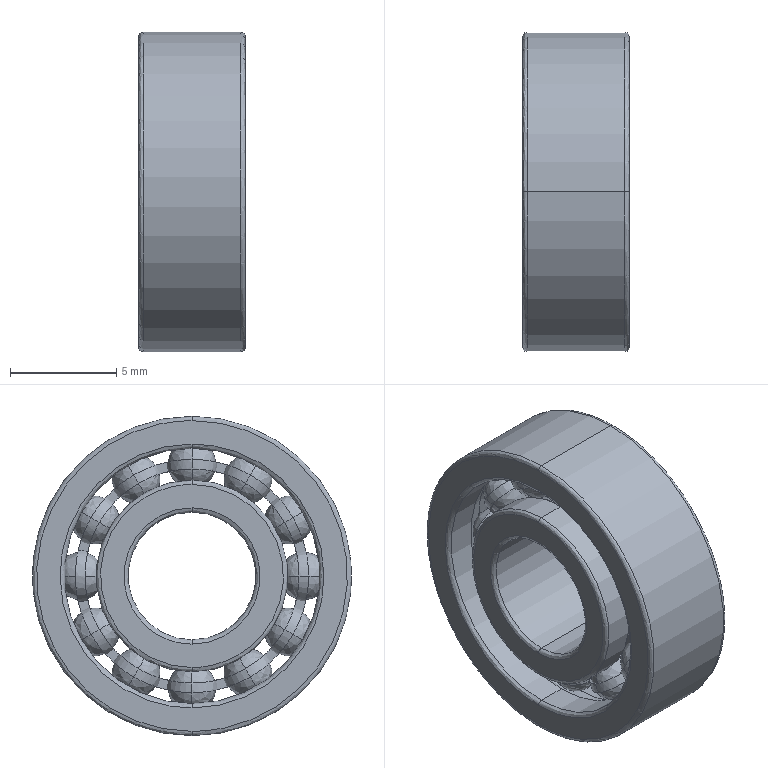Part | SolidWorks | features BaseBody 14 | 14 solids | 159 faces | box 5 x 15 x 15 mm | volume 545.791 mm3 | spline 73 | cylinder 58 | plane 28 | commonest cylinder face diameters 10.05 x23 10.95 x23 9 x4 12 x4 6 x2 15 x2